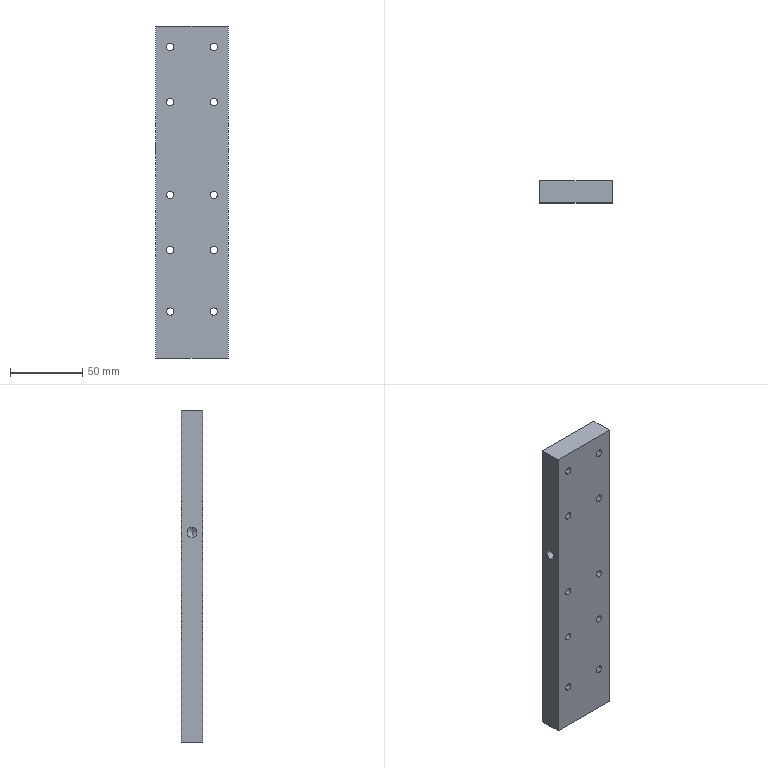Part | 1 solid | 38 faces | box 50 x 15 x 229 mm | volume 166833 mm3 | cylinder 26 | cone 6 | plane 6 | commonest cylinder face diameters 5 x20 6.8 x6
STEP:
#1=CARTESIAN_POINT('',(15.,0.,-48.5));
#2=VERTEX_POINT('',#1);
#3=CARTESIAN_POINT('',(15.,0.,-43.5));
#4=VERTEX_POINT('',#3);
#5=CARTESIAN_POINT('',(15.,0.,-46.));
#6=DIRECTION('',(0.,1.,0.));
#7=DIRECTION('',(0.,0.,1.));
#8=AXIS2_PLACEMENT_3D('',#5,#6,#7);
#9=CIRCLE('',#8,2.5);
#10=EDGE_CURVE('',#2,#4,#9,.T.);
#11=ORIENTED_EDGE('',*,*,#10,.F.);
#12=CARTESIAN_POINT('',(15.,15.,-48.5));
#13=VERTEX_POINT('',#12);
#14=CARTESIAN_POINT('',(15.,15.,-48.5));
#15=DIRECTION('',(0.,1.,0.));
#16=VECTOR('',#15,1000.);
#17=LINE('',#14,#16);
#18=EDGE_CURVE('',#2,#13,#17,.T.);
#19=ORIENTED_EDGE('',*,*,#18,.T.);
#20=CARTESIAN_POINT('',(15.,15.,-43.5));
#21=VERTEX_POINT('',#20);
#22=CARTESIAN_POINT('',(15.,15.,-46.));
#23=DIRECTION('',(0.,1.,0.));
#24=DIRECTION('',(0.,0.,1.));
#25=AXIS2_PLACEMENT_3D('',#22,#23,#24);
#26=CIRCLE('',#25,2.5);
#27=EDGE_CURVE('',#13,#21,#26,.T.);
#28=ORIENTED_EDGE('',*,*,#27,.T.);
#29=CARTESIAN_POINT('',(15.,15.,-43.5));
#30=DIRECTION('',(0.,1.,0.));
#31=VECTOR('',#30,1000.);
#32=LINE('',#29,#31);
#33=EDGE_CURVE('',#4,#21,#32,.T.);
#34=ORIENTED_EDGE('',*,*,#33,.F.);
#35=EDGE_LOOP('',(#11,#19,#28,#34));
#36=FACE_OUTER_BOUND('',#35,.T.);
#37=CARTESIAN_POINT('',(15.,15.,-46.));
#38=DIRECTION('',(0.,1.,0.));
#39=DIRECTION('',(0.,0.,1.));
#40=AXIS2_PLACEMENT_3D('',#37,#38,#39);
#41=CYLINDRICAL_SURFACE('',#40,2.5);
#42=ADVANCED_FACE('',(#36),#41,.F.);
#43=CARTESIAN_POINT('',(-15.,0.,-48.5));
#44=VERTEX_POINT('',#43);
#45=CARTESIAN_POINT('',(-15.,0.,-43.5));
#46=VERTEX_POINT('',#45);
#47=CARTESIAN_POINT('',(-15.,0.,-46.));
#48=DIRECTION('',(0.,1.,0.));
#49=DIRECTION('',(0.,0.,1.));
#50=AXIS2_PLACEMENT_3D('',#47,#48,#49);
#51=CIRCLE('',#50,2.5);
#52=EDGE_CURVE('',#44,#46,#51,.T.);
#53=ORIENTED_EDGE('',*,*,#52,.F.);
#54=CARTESIAN_POINT('',(-15.,15.,-48.5));
#55=VERTEX_POINT('',#54);
#56=CARTESIAN_POINT('',(-15.,15.,-48.5));
#57=DIRECTION('',(0.,1.,0.));
#58=VECTOR('',#57,1000.);
#59=LINE('',#56,#58);
#60=EDGE_CURVE('',#44,#55,#59,.T.);
#61=ORIENTED_EDGE('',*,*,#60,.T.);
#62=CARTESIAN_POINT('',(-15.,15.,-43.5));
#63=VERTEX_POINT('',#62);
#64=CARTESIAN_POINT('',(-15.,15.,-46.));
#65=DIRECTION('',(0.,1.,0.));
#66=DIRECTION('',(0.,0.,1.));
#67=AXIS2_PLACEMENT_3D('',#64,#65,#66);
#68=CIRCLE('',#67,2.5);
#69=EDGE_CURVE('',#55,#63,#68,.T.);
#70=ORIENTED_EDGE('',*,*,#69,.T.);
#71=CARTESIAN_POINT('',(-15.,15.,-43.5));
#72=DIRECTION('',(0.,1.,0.));
#73=VECTOR('',#72,1000.);
#74=LINE('',#71,#73);
#75=EDGE_CURVE('',#46,#63,#74,.T.);
#76=ORIENTED_EDGE('',*,*,#75,.F.);
#77=EDGE_LOOP('',(#53,#61,#70,#76));
#78=FACE_OUTER_BOUND('',#77,.T.);
#79=CARTESIAN_POINT('',(-15.,15.,-46.));
#80=DIRECTION('',(0.,1.,0.));
#81=DIRECTION('',(0.,0.,1.));
#82=AXIS2_PLACEMENT_3D('',#79,#80,#81);
#83=CYLINDRICAL_SURFACE('',#82,2.5);
#84=ADVANCED_FACE('',(#78),#83,.F.);
#85=CARTESIAN_POINT('',(-15.,0.,-10.5));
#86=VERTEX_POINT('',#85);
#87=CARTESIAN_POINT('',(-15.,0.,-5.5));
#88=VERTEX_POINT('',#87);
#89=CARTESIAN_POINT('',(-15.,0.,-8.));
#90=DIRECTION('',(0.,1.,0.));
#91=DIRECTION('',(0.,0.,1.));
#92=AXIS2_PLACEMENT_3D('',#89,#90,#91);
#93=CIRCLE('',#92,2.5);
#94=EDGE_CURVE('',#86,#88,#93,.T.);
#95=ORIENTED_EDGE('',*,*,#94,.F.);
#96=CARTESIAN_POINT('',(-15.,15.,-10.5));
#97=VERTEX_POINT('',#96);
#98=CARTESIAN_POINT('',(-15.,15.,-10.5));
#99=DIRECTION('',(0.,1.,0.));
#100=VECTOR('',#99,1000.);
#101=LINE('',#98,#100);
#102=EDGE_CURVE('',#86,#97,#101,.T.);
#103=ORIENTED_EDGE('',*,*,#102,.T.);
#104=CARTESIAN_POINT('',(-15.,15.,-5.5));
#105=VERTEX_POINT('',#104);
#106=CARTESIAN_POINT('',(-15.,15.,-8.));
#107=DIRECTION('',(0.,1.,0.));
#108=DIRECTION('',(0.,0.,1.));
#109=AXIS2_PLACEMENT_3D('',#106,#107,#108);
#110=CIRCLE('',#109,2.5);
#111=EDGE_CURVE('',#97,#105,#110,.T.);
#112=ORIENTED_EDGE('',*,*,#111,.T.);
#113=CARTESIAN_POINT('',(-15.,15.,-5.5));
#114=DIRECTION('',(0.,1.,0.));
#115=VECTOR('',#114,1000.);
#116=LINE('',#113,#115);
#117=EDGE_CURVE('',#88,#105,#116,.T.);
#118=ORIENTED_EDGE('',*,*,#117,.F.);
#119=EDGE_LOOP('',(#95,#103,#112,#118));
#120=FACE_OUTER_BOUND('',#119,.T.);
#121=CARTESIAN_POINT('',(-15.,15.,-8.));
#122=DIRECTION('',(0.,1.,0.));
#123=DIRECTION('',(0.,0.,1.));
#124=AXIS2_PLACEMENT_3D('',#121,#122,#123);
#125=CYLINDRICAL_SURFACE('',#124,2.5);
#126=ADVANCED_FACE('',(#120),#125,.F.);
#127=CARTESIAN_POINT('',(15.,0.,-10.5));
#128=VERTEX_POINT('',#127);
#129=CARTESIAN_POINT('',(15.,0.,-5.5));
#130=VERTEX_POINT('',#129);
#131=CARTESIAN_POINT('',(15.,0.,-8.));
#132=DIRECTION('',(0.,1.,0.));
#133=DIRECTION('',(0.,0.,1.));
#134=AXIS2_PLACEMENT_3D('',#131,#132,#133);
#135=CIRCLE('',#134,2.5);
#136=EDGE_CURVE('',#128,#130,#135,.T.);
#137=ORIENTED_EDGE('',*,*,#136,.F.);
#138=CARTESIAN_POINT('',(15.,15.,-10.5));
#139=VERTEX_POINT('',#138);
#140=CARTESIAN_POINT('',(15.,15.,-10.5));
#141=DIRECTION('',(0.,1.,0.));
#142=VECTOR('',#141,1000.);
#143=LINE('',#140,#142);
#144=EDGE_CURVE('',#128,#139,#143,.T.);
#145=ORIENTED_EDGE('',*,*,#144,.T.);
#146=CARTESIAN_POINT('',(15.,15.,-5.5));
#147=VERTEX_POINT('',#146);
#148=CARTESIAN_POINT('',(15.,15.,-8.));
#149=DIRECTION('',(0.,1.,0.));
#150=DIRECTION('',(0.,0.,1.));
#151=AXIS2_PLACEMENT_3D('',#148,#149,#150);
#152=CIRCLE('',#151,2.5);
#153=EDGE_CURVE('',#139,#147,#152,.T.);
#154=ORIENTED_EDGE('',*,*,#153,.T.);
#155=CARTESIAN_POINT('',(15.,15.,-5.5));
#156=DIRECTION('',(0.,1.,0.));
#157=VECTOR('',#156,1000.);
#158=LINE('',#155,#157);
#159=EDGE_CURVE('',#130,#147,#158,.T.);
#160=ORIENTED_EDGE('',*,*,#159,.F.);
#161=EDGE_LOOP('',(#137,#145,#154,#160));
#162=FACE_OUTER_BOUND('',#161,.T.);
#163=CARTESIAN_POINT('',(15.,15.,-8.));
#164=DIRECTION('',(0.,1.,0.));
#165=DIRECTION('',(0.,0.,1.));
#166=AXIS2_PLACEMENT_3D('',#163,#164,#165);
#167=CYLINDRICAL_SURFACE('',#166,2.5);
#168=ADVANCED_FACE('',(#162),#167,.F.);
#169=CARTESIAN_POINT('',(15.,0.,53.5));
#170=VERTEX_POINT('',#169);
#171=CARTESIAN_POINT('',(15.,0.,58.5));
#172=VERTEX_POINT('',#171);
#173=CARTESIAN_POINT('',(15.,0.,56.));
#174=DIRECTION('',(0.,1.,0.));
#175=DIRECTION('',(0.,0.,1.));
#176=AXIS2_PLACEMENT_3D('',#173,#174,#175);
#177=CIRCLE('',#176,2.5);
#178=EDGE_CURVE('',#170,#172,#177,.T.);
#179=ORIENTED_EDGE('',*,*,#178,.F.);
#180=CARTESIAN_POINT('',(15.,15.,53.5));
#181=VERTEX_POINT('',#180);
#182=CARTESIAN_POINT('',(15.,15.,53.5));
#183=DIRECTION('',(0.,1.,0.));
#184=VECTOR('',#183,1000.);
#185=LINE('',#182,#184);
#186=EDGE_CURVE('',#170,#181,#185,.T.);
#187=ORIENTED_EDGE('',*,*,#186,.T.);
#188=CARTESIAN_POINT('',(15.,15.,58.5));
#189=VERTEX_POINT('',#188);
#190=CARTESIAN_POINT('',(15.,15.,56.));
#191=DIRECTION('',(0.,1.,0.));
#192=DIRECTION('',(0.,0.,1.));
#193=AXIS2_PLACEMENT_3D('',#190,#191,#192);
#194=CIRCLE('',#193,2.5);
#195=EDGE_CURVE('',#181,#189,#194,.T.);
#196=ORIENTED_EDGE('',*,*,#195,.T.);
#197=CARTESIAN_POINT('',(15.,15.,58.5));
#198=DIRECTION('',(0.,1.,0.));
#199=VECTOR('',#198,1000.);
#200=LINE('',#197,#199);
#201=EDGE_CURVE('',#172,#189,#200,.T.);
#202=ORIENTED_EDGE('',*,*,#201,.F.);
#203=EDGE_LOOP('',(#179,#187,#196,#202));
#204=FACE_OUTER_BOUND('',#203,.T.);
#205=CARTESIAN_POINT('',(15.,15.,56.));
#206=DIRECTION('',(0.,1.,0.));
#207=DIRECTION('',(0.,0.,1.));
#208=AXIS2_PLACEMENT_3D('',#205,#206,#207);
#209=CYLINDRICAL_SURFACE('',#208,2.5);
#210=ADVANCED_FACE('',(#204),#209,.F.);
#211=CARTESIAN_POINT('',(-15.,0.,53.5));
#212=VERTEX_POINT('',#211);
#213=CARTESIAN_POINT('',(-15.,0.,58.5));
#214=VERTEX_POINT('',#213);
#215=CARTESIAN_POINT('',(-15.,0.,56.));
#216=DIRECTION('',(0.,1.,0.));
#217=DIRECTION('',(0.,0.,1.));
#218=AXIS2_PLACEMENT_3D('',#215,#216,#217);
#219=CIRCLE('',#218,2.5);
#220=EDGE_CURVE('',#212,#214,#219,.T.);
#221=ORIENTED_EDGE('',*,*,#220,.F.);
#222=CARTESIAN_POINT('',(-15.,15.,53.5));
#223=VERTEX_POINT('',#222);
#224=CARTESIAN_POINT('',(-15.,15.,53.5));
#225=DIRECTION('',(0.,1.,0.));
#226=VECTOR('',#225,1000.);
#227=LINE('',#224,#226);
#228=EDGE_CURVE('',#212,#223,#227,.T.);
#229=ORIENTED_EDGE('',*,*,#228,.T.);
#230=CARTESIAN_POINT('',(-15.,15.,58.5));
#231=VERTEX_POINT('',#230);
#232=CARTESIAN_POINT('',(-15.,15.,56.));
#233=DIRECTION('',(0.,1.,0.));
#234=DIRECTION('',(0.,0.,1.));
#235=AXIS2_PLACEMENT_3D('',#232,#233,#234);
#236=CIRCLE('',#235,2.5);
#237=EDGE_CURVE('',#223,#231,#236,.T.);
#238=ORIENTED_EDGE('',*,*,#237,.T.);
#239=CARTESIAN_POINT('',(-15.,15.,58.5));
#240=DIRECTION('',(0.,1.,0.));
#241=VECTOR('',#240,1000.);
#242=LINE('',#239,#241);
#243=EDGE_CURVE('',#214,#231,#242,.T.);
#244=ORIENTED_EDGE('',*,*,#243,.F.);
#245=EDGE_LOOP('',(#221,#229,#238,#244));
#246=FACE_OUTER_BOUND('',#245,.T.);
#247=CARTESIAN_POINT('',(-15.,15.,56.));
#248=DIRECTION('',(0.,1.,0.));
#249=DIRECTION('',(0.,0.,1.));
#250=AXIS2_PLACEMENT_3D('',#247,#248,#249);
#251=CYLINDRICAL_SURFACE('',#250,2.5);
#252=ADVANCED_FACE('',(#246),#251,.F.);
#253=CARTESIAN_POINT('',(15.,0.,91.5));
#254=VERTEX_POINT('',#253);
#255=CARTESIAN_POINT('',(15.,0.,96.5));
#256=VERTEX_POINT('',#255);
#257=CARTESIAN_POINT('',(15.,0.,94.));
#258=DIRECTION('',(0.,1.,0.));
#259=DIRECTION('',(0.,0.,1.));
#260=AXIS2_PLACEMENT_3D('',#257,#258,#259);
#261=CIRCLE('',#260,2.5);
#262=EDGE_CURVE('',#254,#256,#261,.T.);
#263=ORIENTED_EDGE('',*,*,#262,.F.);
#264=CARTESIAN_POINT('',(15.,15.,91.5));
#265=VERTEX_POINT('',#264);
#266=CARTESIAN_POINT('',(15.,15.,91.5));
#267=DIRECTION('',(0.,1.,0.));
#268=VECTOR('',#267,1000.);
#269=LINE('',#266,#268);
#270=EDGE_CURVE('',#254,#265,#269,.T.);
#271=ORIENTED_EDGE('',*,*,#270,.T.);
#272=CARTESIAN_POINT('',(15.,15.,96.5));
#273=VERTEX_POINT('',#272);
#274=CARTESIAN_POINT('',(15.,15.,94.));
#275=DIRECTION('',(0.,1.,0.));
#276=DIRECTION('',(0.,0.,1.));
#277=AXIS2_PLACEMENT_3D('',#274,#275,#276);
#278=CIRCLE('',#277,2.5);
#279=EDGE_CURVE('',#265,#273,#278,.T.);
#280=ORIENTED_EDGE('',*,*,#279,.T.);
#281=CARTESIAN_POINT('',(15.,15.,96.5));
#282=DIRECTION('',(0.,1.,0.));
#283=VECTOR('',#282,1000.);
#284=LINE('',#281,#283);
#285=EDGE_CURVE('',#256,#273,#284,.T.);
#286=ORIENTED_EDGE('',*,*,#285,.F.);
#287=EDGE_LOOP('',(#263,#271,#280,#286));
#288=FACE_OUTER_BOUND('',#287,.T.);
#289=CARTESIAN_POINT('',(15.,15.,94.));
#290=DIRECTION('',(0.,1.,0.));
#291=DIRECTION('',(0.,0.,1.));
#292=AXIS2_PLACEMENT_3D('',#289,#290,#291);
#293=CYLINDRICAL_SURFACE('',#292,2.5);
#294=ADVANCED_FACE('',(#288),#293,.F.);
#295=CARTESIAN_POINT('',(-15.,0.,91.5));
#296=VERTEX_POINT('',#295);
#297=CARTESIAN_POINT('',(-15.,0.,96.5));
#298=VERTEX_POINT('',#297);
#299=CARTESIAN_POINT('',(-15.,0.,94.));
#300=DIRECTION('',(0.,1.,0.));
#301=DIRECTION('',(0.,0.,1.));
#302=AXIS2_PLACEMENT_3D('',#299,#300,#301);
#303=CIRCLE('',#302,2.5);
#304=EDGE_CURVE('',#296,#298,#303,.T.);
#305=ORIENTED_EDGE('',*,*,#304,.F.);
#306=CARTESIAN_POINT('',(-15.,15.,91.5));
#307=VERTEX_POINT('',#306);
#308=CARTESIAN_POINT('',(-15.,15.,91.5));
#309=DIRECTION('',(0.,1.,0.));
#310=VECTOR('',#309,1000.);
#311=LINE('',#308,#310);
#312=EDGE_CURVE('',#296,#307,#311,.T.);
#313=ORIENTED_EDGE('',*,*,#312,.T.);
#314=CARTESIAN_POINT('',(-15.,15.,96.5));
#315=VERTEX_POINT('',#314);
#316=CARTESIAN_POINT('',(-15.,15.,94.));
#317=DIRECTION('',(0.,1.,0.));
#318=DIRECTION('',(0.,0.,1.));
#319=AXIS2_PLACEMENT_3D('',#316,#317,#318);
#320=CIRCLE('',#319,2.5);
#321=EDGE_CURVE('',#307,#315,#320,.T.);
#322=ORIENTED_EDGE('',*,*,#321,.T.);
#323=CARTESIAN_POINT('',(-15.,15.,96.5));
#324=DIRECTION('',(0.,1.,0.));
#325=VECTOR('',#324,1000.);
#326=LINE('',#323,#325);
#327=EDGE_CURVE('',#298,#315,#326,.T.);
#328=ORIENTED_EDGE('',*,*,#327,.F.);
#329=EDGE_LOOP('',(#305,#313,#322,#328));
#330=FACE_OUTER_BOUND('',#329,.T.);
#331=CARTESIAN_POINT('',(-15.,15.,94.));
#332=DIRECTION('',(0.,1.,0.));
#333=DIRECTION('',(0.,0.,1.));
#334=AXIS2_PLACEMENT_3D('',#331,#332,#333);
#335=CYLINDRICAL_SURFACE('',#334,2.5);
#336=ADVANCED_FACE('',(#330),#335,.F.);
#337=CARTESIAN_POINT('',(15.,0.,-91.));
#338=VERTEX_POINT('',#337);
#339=CARTESIAN_POINT('',(15.,0.,-86.));
#340=VERTEX_POINT('',#339);
#341=CARTESIAN_POINT('',(15.,0.,-88.5));
#342=DIRECTION('',(0.,1.,0.));
#343=DIRECTION('',(0.,0.,1.));
#344=AXIS2_PLACEMENT_3D('',#341,#342,#343);
#345=CIRCLE('',#344,2.5);
#346=EDGE_CURVE('',#338,#340,#345,.T.);
#347=ORIENTED_EDGE('',*,*,#346,.F.);
#348=CARTESIAN_POINT('',(15.,15.,-91.));
#349=VERTEX_POINT('',#348);
#350=CARTESIAN_POINT('',(15.,15.,-91.));
#351=DIRECTION('',(0.,1.,0.));
#352=VECTOR('',#351,1000.);
#353=LINE('',#350,#352);
#354=EDGE_CURVE('',#338,#349,#353,.T.);
#355=ORIENTED_EDGE('',*,*,#354,.T.);
#356=CARTESIAN_POINT('',(15.,15.,-86.));
#357=VERTEX_POINT('',#356);
#358=CARTESIAN_POINT('',(15.,15.,-88.5));
#359=DIRECTION('',(0.,1.,0.));
#360=DIRECTION('',(0.,0.,1.));
#361=AXIS2_PLACEMENT_3D('',#358,#359,#360);
#362=CIRCLE('',#361,2.5);
#363=EDGE_CURVE('',#349,#357,#362,.T.);
#364=ORIENTED_EDGE('',*,*,#363,.T.);
#365=CARTESIAN_POINT('',(15.,15.,-86.));
#366=DIRECTION('',(0.,1.,0.));
#367=VECTOR('',#366,1000.);
#368=LINE('',#365,#367);
#369=EDGE_CURVE('',#340,#357,#368,.T.);
#370=ORIENTED_EDGE('',*,*,#369,.F.);
#371=EDGE_LOOP('',(#347,#355,#364,#370));
#372=FACE_OUTER_BOUND('',#371,.T.);
#373=CARTESIAN_POINT('',(15.,15.,-88.5));
#374=DIRECTION('',(0.,1.,0.));
#375=DIRECTION('',(0.,0.,1.));
#376=AXIS2_PLACEMENT_3D('',#373,#374,#375);
#377=CYLINDRICAL_SURFACE('',#376,2.5);
#378=ADVANCED_FACE('',(#372),#377,.F.);
#379=CARTESIAN_POINT('',(-15.,0.,-91.));
#380=VERTEX_POINT('',#379);
#381=CARTESIAN_POINT('',(-15.,0.,-86.));
#382=VERTEX_POINT('',#381);
#383=CARTESIAN_POINT('',(-15.,0.,-88.5));
#384=DIRECTION('',(0.,1.,0.));
#385=DIRECTION('',(0.,0.,1.));
#386=AXIS2_PLACEMENT_3D('',#383,#384,#385);
#387=CIRCLE('',#386,2.5);
#388=EDGE_CURVE('',#380,#382,#387,.T.);
#389=ORIENTED_EDGE('',*,*,#388,.F.);
#390=CARTESIAN_POINT('',(-15.,15.,-91.));
#391=VERTEX_POINT('',#390);
#392=CARTESIAN_POINT('',(-15.,15.,-91.));
#393=DIRECTION('',(0.,1.,0.));
#394=VECTOR('',#393,1000.);
#395=LINE('',#392,#394);
#396=EDGE_CURVE('',#380,#391,#395,.T.);
#397=ORIENTED_EDGE('',*,*,#396,.T.);
#398=CARTESIAN_POINT('',(-15.,15.,-86.));
#399=VERTEX_POINT('',#398);
#400=CARTESIAN_POINT('',(-15.,15.,-88.5));
#401=DIRECTION('',(0.,1.,0.));
#402=DIRECTION('',(0.,0.,1.));
#403=AXIS2_PLACEMENT_3D('',#400,#401,#402);
#404=CIRCLE('',#403,2.5);
#405=EDGE_CURVE('',#391,#399,#404,.T.);
#406=ORIENTED_EDGE('',*,*,#405,.T.);
#407=CARTESIAN_POINT('',(-15.,15.,-86.));
#408=DIRECTION('',(0.,1.,0.));
#409=VECTOR('',#408,1000.);
#410=LINE('',#407,#409);
#411=EDGE_CURVE('',#382,#399,#410,.T.);
#412=ORIENTED_EDGE('',*,*,#411,.F.);
#413=EDGE_LOOP('',(#389,#397,#406,#412));
#414=FACE_OUTER_BOUND('',#413,.T.);
#415=CARTESIAN_POINT('',(-15.,15.,-88.5));
#416=DIRECTION('',(0.,1.,0.));
#417=DIRECTION('',(0.,0.,1.));
#418=AXIS2_PLACEMENT_3D('',#415,#416,#417);
#419=CYLINDRICAL_SURFACE('',#418,2.5);
#420=ADVANCED_FACE('',(#414),#419,.F.);
#421=CARTESIAN_POINT('',(-2.75,7.5,20.7));
#422=VERTEX_POINT('',#421);
#423=CARTESIAN_POINT('',(-2.75,7.5,27.5));
#424=VERTEX_POINT('',#423);
#425=CARTESIAN_POINT('',(-2.75,7.5,24.1));
#426=DIRECTION('',(-1.,0.,0.));
#427=DIRECTION('',(0.,0.,1.));
#428=AXIS2_PLACEMENT_3D('',#425,#426,#427);
#429=CIRCLE('',#428,3.4);
#430=EDGE_CURVE('',#422,#424,#429,.T.);
#431=ORIENTED_EDGE('',*,*,#430,.F.);
#432=CARTESIAN_POINT('',(-25.,7.5,20.7));
#433=VERTEX_POINT('',#432);
#434=CARTESIAN_POINT('',(-25.,7.5,20.7));
#435=DIRECTION('',(-1.,0.,0.));
#436=VECTOR('',#435,1000.);
#437=LINE('',#434,#436);
#438=EDGE_CURVE('',#422,#433,#437,.T.);
#439=ORIENTED_EDGE('',*,*,#438,.T.);
#440=CARTESIAN_POINT('',(-25.,7.5,27.5));
#441=VERTEX_POINT('',#440);
#442=CARTESIAN_POINT('',(-25.,7.5,24.1));
#443=DIRECTION('',(-1.,0.,0.));
#444=DIRECTION('',(0.,0.,1.));
#445=AXIS2_PLACEMENT_3D('',#442,#443,#444);
#446=CIRCLE('',#445,3.4);
#447=EDGE_CURVE('',#433,#441,#446,.T.);
#448=ORIENTED_EDGE('',*,*,#447,.T.);
#449=CARTESIAN_POINT('',(-25.,7.5,27.5));
#450=DIRECTION('',(-1.,0.,0.));
#451=VECTOR('',#450,1000.);
#452=LINE('',#449,#451);
#453=EDGE_CURVE('',#424,#441,#452,.T.);
#454=ORIENTED_EDGE('',*,*,#453,.F.);
#455=EDGE_LOOP('',(#431,#439,#448,#454));
#456=FACE_OUTER_BOUND('',#455,.T.);
#457=CARTESIAN_POINT('',(-25.,7.5,24.1));
#458=DIRECTION('',(-1.,0.,0.));
#459=DIRECTION('',(0.,0.,1.));
#460=AXIS2_PLACEMENT_3D('',#457,#458,#459);
#461=CYLINDRICAL_SURFACE('',#460,3.4);
#462=ADVANCED_FACE('',(#456),#461,.F.);
#463=CARTESIAN_POINT('',(-0.7071,7.5,24.1));
#464=VERTEX_POINT('',#463);
#465=CARTESIAN_POINT('',(-2.75,7.5,27.5));
#466=DIRECTION('',(-0.515,0.,0.8572));
#467=VECTOR('',#466,1000.);
#468=LINE('',#465,#467);
#469=EDGE_CURVE('',#464,#424,#468,.T.);
#470=ORIENTED_EDGE('',*,*,#469,.F.);
#471=CARTESIAN_POINT('',(-2.75,7.5,20.7));
#472=DIRECTION('',(-0.515,0.,-0.8572));
#473=VECTOR('',#472,1000.);
#474=LINE('',#471,#473);
#475=EDGE_CURVE('',#464,#422,#474,.T.);
#476=ORIENTED_EDGE('',*,*,#475,.T.);
#477=ORIENTED_EDGE('',*,*,#430,.T.);
#478=EDGE_LOOP('',(#470,#476,#477));
#479=FACE_OUTER_BOUND('',#478,.T.);
#480=CARTESIAN_POINT('',(-2.75,7.5,24.1));
#481=DIRECTION('',(-1.,0.,0.));
#482=DIRECTION('',(0.,0.,1.));
#483=AXIS2_PLACEMENT_3D('',#480,#481,#482);
#484=CONICAL_SURFACE('',#483,3.4,1.03);
#485=ADVANCED_FACE('',(#479),#484,.F.);
#486=CARTESIAN_POINT('',(-11.6,7.5,-105.5));
#487=VERTEX_POINT('',#486);
#488=CARTESIAN_POINT('',(-18.4,7.5,-105.5));
#489=VERTEX_POINT('',#488);
#490=CARTESIAN_POINT('',(-15.,7.5,-105.5));
#491=DIRECTION('',(0.,0.,-1.));
#492=DIRECTION('',(-1.,0.,0.));
#493=AXIS2_PLACEMENT_3D('',#490,#491,#492);
#494=CIRCLE('',#493,3.4);
#495=EDGE_CURVE('',#487,#489,#494,.T.);
#496=ORIENTED_EDGE('',*,*,#495,.F.);
#497=CARTESIAN_POINT('',(-11.6,7.5,-120.5));
#498=VERTEX_POINT('',#497);
#499=CARTESIAN_POINT('',(-11.6,7.5,-120.5));
#500=DIRECTION('',(0.,0.,-1.));
#501=VECTOR('',#500,1000.);
#502=LINE('',#499,#501);
#503=EDGE_CURVE('',#487,#498,#502,.T.);
#504=ORIENTED_EDGE('',*,*,#503,.T.);
#505=CARTESIAN_POINT('',(-18.4,7.5,-120.5));
#506=VERTEX_POINT('',#505);
#507=CARTESIAN_POINT('',(-15.,7.5,-120.5));
#508=DIRECTION('',(0.,0.,-1.));
#509=DIRECTION('',(-1.,0.,0.));
#510=AXIS2_PLACEMENT_3D('',#507,#508,#509);
#511=CIRCLE('',#510,3.4);
#512=EDGE_CURVE('',#498,#506,#511,.T.);
#513=ORIENTED_EDGE('',*,*,#512,.T.);
#514=CARTESIAN_POINT('',(-18.4,7.5,-120.5));
#515=DIRECTION('',(0.,0.,-1.));
#516=VECTOR('',#515,1000.);
#517=LINE('',#514,#516);
#518=EDGE_CURVE('',#489,#506,#517,.T.);
#519=ORIENTED_EDGE('',*,*,#518,.F.);
#520=EDGE_LOOP('',(#496,#504,#513,#519));
#521=FACE_OUTER_BOUND('',#520,.T.);
#522=CARTESIAN_POINT('',(-15.,7.5,-120.5));
#523=DIRECTION('',(0.,0.,-1.));
#524=DIRECTION('',(-1.,0.,0.));
#525=AXIS2_PLACEMENT_3D('',#522,#523,#524);
#526=CYLINDRICAL_SURFACE('',#525,3.4);
#527=ADVANCED_FACE('',(#521),#526,.F.);
#528=CARTESIAN_POINT('',(-15.,7.5,-103.457));
#529=VERTEX_POINT('',#528);
#530=CARTESIAN_POINT('',(-18.4,7.5,-105.5));
#531=DIRECTION('',(-0.8572,0.,-0.515));
#532=VECTOR('',#531,1000.);
#533=LINE('',#530,#532);
#534=EDGE_CURVE('',#529,#489,#533,.T.);
#535=ORIENTED_EDGE('',*,*,#534,.F.);
#536=CARTESIAN_POINT('',(-11.6,7.5,-105.5));
#537=DIRECTION('',(0.8572,0.,-0.515));
#538=VECTOR('',#537,1000.);
#539=LINE('',#536,#538);
#540=EDGE_CURVE('',#529,#487,#539,.T.);
#541=ORIENTED_EDGE('',*,*,#540,.T.);
#542=ORIENTED_EDGE('',*,*,#495,.T.);
#543=EDGE_LOOP('',(#535,#541,#542));
#544=FACE_OUTER_BOUND('',#543,.T.);
#545=CARTESIAN_POINT('',(-15.,7.5,-105.5));
#546=DIRECTION('',(0.,0.,-1.));
#547=DIRECTION('',(-1.,0.,0.));
#548=AXIS2_PLACEMENT_3D('',#545,#546,#547);
#549=CONICAL_SURFACE('',#548,3.4,1.03);
#550=ADVANCED_FACE('',(#544),#549,.F.);
#551=CARTESIAN_POINT('',(18.4,7.5,-105.5));
#552=VERTEX_POINT('',#551);
#553=CARTESIAN_POINT('',(11.6,7.5,-105.5));
#554=VERTEX_POINT('',#553);
#555=CARTESIAN_POINT('',(15.,7.5,-105.5));
#556=DIRECTION('',(0.,0.,-1.));
#557=DIRECTION('',(-1.,0.,0.));
#558=AXIS2_PLACEMENT_3D('',#555,#556,#557);
#559=CIRCLE('',#558,3.4);
#560=EDGE_CURVE('',#552,#554,#559,.T.);
#561=ORIENTED_EDGE('',*,*,#560,.F.);
#562=CARTESIAN_POINT('',(18.4,7.5,-120.5));
#563=VERTEX_POINT('',#562);
#564=CARTESIAN_POINT('',(18.4,7.5,-120.5));
#565=DIRECTION('',(0.,0.,-1.));
#566=VECTOR('',#565,1000.);
#567=LINE('',#564,#566);
#568=EDGE_CURVE('',#552,#563,#567,.T.);
#569=ORIENTED_EDGE('',*,*,#568,.T.);
#570=CARTESIAN_POINT('',(11.6,7.5,-120.5));
#571=VERTEX_POINT('',#570);
#572=CARTESIAN_POINT('',(15.,7.5,-120.5));
#573=DIRECTION('',(0.,0.,-1.));
#574=DIRECTION('',(-1.,0.,0.));
#575=AXIS2_PLACEMENT_3D('',#572,#573,#574);
#576=CIRCLE('',#575,3.4);
#577=EDGE_CURVE('',#563,#571,#576,.T.);
#578=ORIENTED_EDGE('',*,*,#577,.T.);
#579=CARTESIAN_POINT('',(11.6,7.5,-120.5));
#580=DIRECTION('',(0.,0.,-1.));
#581=VECTOR('',#580,1000.);
#582=LINE('',#579,#581);
#583=EDGE_CURVE('',#554,#571,#582,.T.);
#584=ORIENTED_EDGE('',*,*,#583,.F.);
#585=EDGE_LOOP('',(#561,#569,#578,#584));
#586=FACE_OUTER_BOUND('',#585,.T.);
#587=CARTESIAN_POINT('',(15.,7.5,-120.5));
#588=DIRECTION('',(0.,0.,-1.));
#589=DIRECTION('',(-1.,0.,0.));
#590=AXIS2_PLACEMENT_3D('',#587,#588,#589);
#591=CYLINDRICAL_SURFACE('',#590,3.4);
#592=ADVANCED_FACE('',(#586),#591,.F.);
#593=CARTESIAN_POINT('',(15.,7.5,-103.457));
#594=VERTEX_POINT('',#593);
#595=CARTESIAN_POINT('',(11.6,7.5,-105.5));
#596=DIRECTION('',(-0.8572,0.,-0.515));
#597=VECTOR('',#596,1000.);
#598=LINE('',#595,#597);
#599=EDGE_CURVE('',#594,#554,#598,.T.);
#600=ORIENTED_EDGE('',*,*,#599,.F.);
#601=CARTESIAN_POINT('',(18.4,7.5,-105.5));
#602=DIRECTION('',(0.8572,0.,-0.515));
#603=VECTOR('',#602,1000.);
#604=LINE('',#601,#603);
#605=EDGE_CURVE('',#594,#552,#604,.T.);
#606=ORIENTED_EDGE('',*,*,#605,.T.);
#607=ORIENTED_EDGE('',*,*,#560,.T.);
#608=EDGE_LOOP('',(#600,#606,#607));
#609=FACE_OUTER_BOUND('',#608,.T.);
#610=CARTESIAN_POINT('',(15.,7.5,-105.5));
#611=DIRECTION('',(0.,0.,-1.));
#612=DIRECTION('',(-1.,0.,0.));
#613=AXIS2_PLACEMENT_3D('',#610,#611,#612);
#614=CONICAL_SURFACE('',#613,3.4,1.03);
#615=ADVANCED_FACE('',(#609),#614,.F.);
#616=CARTESIAN_POINT('',(-25.,15.,108.5));
#617=VERTEX_POINT('',#616);
#618=CARTESIAN_POINT('',(25.,15.,108.5));
#619=VERTEX_POINT('',#618);
#620=CARTESIAN_POINT('',(-25.,15.,108.5));
#621=DIRECTION('',(1.,0.,0.));
#622=VECTOR('',#621,1000.);
#623=LINE('',#620,#622);
#624=EDGE_CURVE('',#617,#619,#623,.T.);
#625=ORIENTED_EDGE('',*,*,#624,.F.);
#626=CARTESIAN_POINT('',(-25.,0.,108.5));
#627=VERTEX_POINT('',#626);
#628=CARTESIAN_POINT('',(-25.,0.,108.5));
#629=DIRECTION('',(0.,1.,0.));
#630=VECTOR('',#629,1000.);
#631=LINE('',#628,#630);
#632=EDGE_CURVE('',#627,#617,#631,.T.);
#633=ORIENTED_EDGE('',*,*,#632,.F.);
#634=CARTESIAN_POINT('',(25.,0.,108.5));
#635=VERTEX_POINT('',#634);
#636=CARTESIAN_POINT('',(-25.,0.,108.5));
#637=DIRECTION('',(1.,0.,0.));
#638=VECTOR('',#637,1000.);
#639=LINE('',#636,#638);
#640=EDGE_CURVE('',#627,#635,#639,.T.);
#641=ORIENTED_EDGE('',*,*,#640,.T.);
#642=CARTESIAN_POINT('',(25.,0.,108.5));
#643=DIRECTION('',(0.,1.,0.));
#644=VECTOR('',#643,1000.);
#645=LINE('',#642,#644);
#646=EDGE_CURVE('',#635,#619,#645,.T.);
#647=ORIENTED_EDGE('',*,*,#646,.T.);
#648=EDGE_LOOP('',(#625,#633,#641,#647));
#649=FACE_OUTER_BOUND('',#648,.T.);
#650=CARTESIAN_POINT('',(-25.,0.,108.5));
#651=DIRECTION('',(0.,0.,1.));
#652=DIRECTION('',(1.,0.,0.));
#653=AXIS2_PLACEMENT_3D('',#650,#651,#652);
#654=PLANE('',#653);
#655=ADVANCED_FACE('',(#649),#654,.T.);
#656=CARTESIAN_POINT('',(-25.,7.5,24.1));
#657=DIRECTION('',(-1.,0.,0.));
#658=DIRECTION('',(0.,0.,1.));
#659=AXIS2_PLACEMENT_3D('',#656,#657,#658);
#660=CIRCLE('',#659,3.4);
#661=EDGE_CURVE('',#441,#433,#660,.T.);
#662=ORIENTED_EDGE('',*,*,#661,.F.);
#663=ORIENTED_EDGE('',*,*,#447,.F.);
#664=EDGE_LOOP('',(#662,#663));
#665=FACE_BOUND('',#664,.T.);
#666=CARTESIAN_POINT('',(-25.,15.,-120.5));
#667=VERTEX_POINT('',#666);
#668=CARTESIAN_POINT('',(-25.,15.,-120.5));
#669=DIRECTION('',(0.,0.,1.));
#670=VECTOR('',#669,1000.);
#671=LINE('',#668,#670);
#672=EDGE_CURVE('',#667,#617,#671,.T.);
#673=ORIENTED_EDGE('',*,*,#672,.F.);
#674=CARTESIAN_POINT('',(-25.,0.,-120.5));
#675=VERTEX_POINT('',#674);
#676=CARTESIAN_POINT('',(-25.,0.,-120.5));
#677=DIRECTION('',(0.,1.,0.));
#678=VECTOR('',#677,1000.);
#679=LINE('',#676,#678);
#680=EDGE_CURVE('',#675,#667,#679,.T.);
#681=ORIENTED_EDGE('',*,*,#680,.F.);
#682=CARTESIAN_POINT('',(-25.,0.,-120.5));
#683=DIRECTION('',(0.,0.,1.));
#684=VECTOR('',#683,1000.);
#685=LINE('',#682,#684);
#686=EDGE_CURVE('',#675,#627,#685,.T.);
#687=ORIENTED_EDGE('',*,*,#686,.T.);
#688=ORIENTED_EDGE('',*,*,#632,.T.);
#689=EDGE_LOOP('',(#673,#681,#687,#688));
#690=FACE_OUTER_BOUND('',#689,.T.);
#691=CARTESIAN_POINT('',(-25.,0.,-120.5));
#692=DIRECTION('',(-1.,0.,0.));
#693=DIRECTION('',(0.,0.,1.));
#694=AXIS2_PLACEMENT_3D('',#691,#692,#693);
#695=PLANE('',#694);
#696=ADVANCED_FACE('',(#665,#690),#695,.T.);
#697=CARTESIAN_POINT('',(-15.,7.5,-120.5));
#698=DIRECTION('',(0.,0.,-1.));
#699=DIRECTION('',(-1.,0.,0.));
#700=AXIS2_PLACEMENT_3D('',#697,#698,#699);
#701=CIRCLE('',#700,3.4);
#702=EDGE_CURVE('',#506,#498,#701,.T.);
#703=ORIENTED_EDGE('',*,*,#702,.F.);
#704=ORIENTED_EDGE('',*,*,#512,.F.);
#705=EDGE_LOOP('',(#703,#704));
#706=FACE_BOUND('',#705,.T.);
#707=CARTESIAN_POINT('',(15.,7.5,-120.5));
#708=DIRECTION('',(0.,0.,-1.));
#709=DIRECTION('',(-1.,0.,0.));
#710=AXIS2_PLACEMENT_3D('',#707,#708,#709);
#711=CIRCLE('',#710,3.4);
#712=EDGE_CURVE('',#571,#563,#711,.T.);
#713=ORIENTED_EDGE('',*,*,#712,.F.);
#714=ORIENTED_EDGE('',*,*,#577,.F.);
#715=EDGE_LOOP('',(#713,#714));
#716=FACE_BOUND('',#715,.T.);
#717=CARTESIAN_POINT('',(25.,15.,-120.5));
#718=VERTEX_POINT('',#717);
#719=CARTESIAN_POINT('',(25.,15.,-120.5));
#720=DIRECTION('',(-1.,0.,0.));
#721=VECTOR('',#720,1000.);
#722=LINE('',#719,#721);
#723=EDGE_CURVE('',#718,#667,#722,.T.);
#724=ORIENTED_EDGE('',*,*,#723,.F.);
#725=CARTESIAN_POINT('',(25.,0.,-120.5));
#726=VERTEX_POINT('',#725);
#727=CARTESIAN_POINT('',(25.,0.,-120.5));
#728=DIRECTION('',(0.,1.,0.));
#729=VECTOR('',#728,1000.);
#730=LINE('',#727,#729);
#731=EDGE_CURVE('',#726,#718,#730,.T.);
#732=ORIENTED_EDGE('',*,*,#731,.F.);
#733=CARTESIAN_POINT('',(25.,0.,-120.5));
#734=DIRECTION('',(-1.,0.,0.));
#735=VECTOR('',#734,1000.);
#736=LINE('',#733,#735);
#737=EDGE_CURVE('',#726,#675,#736,.T.);
#738=ORIENTED_EDGE('',*,*,#737,.T.);
#739=ORIENTED_EDGE('',*,*,#680,.T.);
#740=EDGE_LOOP('',(#724,#732,#738,#739));
#741=FACE_OUTER_BOUND('',#740,.T.);
#742=CARTESIAN_POINT('',(25.,0.,-120.5));
#743=DIRECTION('',(0.,0.,-1.));
#744=DIRECTION('',(-1.,0.,0.));
#745=AXIS2_PLACEMENT_3D('',#742,#743,#744);
#746=PLANE('',#745);
#747=ADVANCED_FACE('',(#706,#716,#741),#746,.T.);
#748=CARTESIAN_POINT('',(25.,15.,108.5));
#749=DIRECTION('',(0.,0.,-1.));
#750=VECTOR('',#749,1000.);
#751=LINE('',#748,#750);
#752=EDGE_CURVE('',#619,#718,#751,.T.);
#753=ORIENTED_EDGE('',*,*,#752,.F.);
#754=ORIENTED_EDGE('',*,*,#646,.F.);
#755=CARTESIAN_POINT('',(25.,0.,108.5));
#756=DIRECTION('',(0.,0.,-1.));
#757=VECTOR('',#756,1000.);
#758=LINE('',#755,#757);
#759=EDGE_CURVE('',#635,#726,#758,.T.);
#760=ORIENTED_EDGE('',*,*,#759,.T.);
#761=ORIENTED_EDGE('',*,*,#731,.T.);
#762=EDGE_LOOP('',(#753,#754,#760,#761));
#763=FACE_OUTER_BOUND('',#762,.T.);
#764=CARTESIAN_POINT('',(25.,0.,108.5));
#765=DIRECTION('',(1.,0.,0.));
#766=DIRECTION('',(0.,0.,-1.));
#767=AXIS2_PLACEMENT_3D('',#764,#765,#766);
#768=PLANE('',#767);
#769=ADVANCED_FACE('',(#763),#768,.T.);
#770=CARTESIAN_POINT('',(15.,0.,-46.));
#771=DIRECTION('',(0.,1.,0.));
#772=DIRECTION('',(0.,0.,1.));
#773=AXIS2_PLACEMENT_3D('',#770,#771,#772);
#774=CIRCLE('',#773,2.5);
#775=EDGE_CURVE('',#4,#2,#774,.T.);
#776=ORIENTED_EDGE('',*,*,#775,.T.);
#777=ORIENTED_EDGE('',*,*,#10,.T.);
#778=EDGE_LOOP('',(#776,#777));
#779=FACE_BOUND('',#778,.T.);
#780=CARTESIAN_POINT('',(-15.,0.,-46.));
#781=DIRECTION('',(0.,1.,0.));
#782=DIRECTION('',(0.,0.,1.));
#783=AXIS2_PLACEMENT_3D('',#780,#781,#782);
#784=CIRCLE('',#783,2.5);
#785=EDGE_CURVE('',#46,#44,#784,.T.);
#786=ORIENTED_EDGE('',*,*,#785,.T.);
#787=ORIENTED_EDGE('',*,*,#52,.T.);
#788=EDGE_LOOP('',(#786,#787));
#789=FACE_BOUND('',#788,.T.);
#790=CARTESIAN_POINT('',(-15.,0.,-8.));
#791=DIRECTION('',(0.,1.,0.));
#792=DIRECTION('',(0.,0.,1.));
#793=AXIS2_PLACEMENT_3D('',#790,#791,#792);
#794=CIRCLE('',#793,2.5);
#795=EDGE_CURVE('',#88,#86,#794,.T.);
#796=ORIENTED_EDGE('',*,*,#795,.T.);
#797=ORIENTED_EDGE('',*,*,#94,.T.);
#798=EDGE_LOOP('',(#796,#797));
#799=FACE_BOUND('',#798,.T.);
#800=CARTESIAN_POINT('',(15.,0.,-8.));
#801=DIRECTION('',(0.,1.,0.));
#802=DIRECTION('',(0.,0.,1.));
#803=AXIS2_PLACEMENT_3D('',#800,#801,#802);
#804=CIRCLE('',#803,2.5);
#805=EDGE_CURVE('',#130,#128,#804,.T.);
#806=ORIENTED_EDGE('',*,*,#805,.T.);
#807=ORIENTED_EDGE('',*,*,#136,.T.);
#808=EDGE_LOOP('',(#806,#807));
#809=FACE_BOUND('',#808,.T.);
#810=CARTESIAN_POINT('',(15.,0.,56.));
#811=DIRECTION('',(0.,1.,0.));
#812=DIRECTION('',(0.,0.,1.));
#813=AXIS2_PLACEMENT_3D('',#810,#811,#812);
#814=CIRCLE('',#813,2.5);
#815=EDGE_CURVE('',#172,#170,#814,.T.);
#816=ORIENTED_EDGE('',*,*,#815,.T.);
#817=ORIENTED_EDGE('',*,*,#178,.T.);
#818=EDGE_LOOP('',(#816,#817));
#819=FACE_BOUND('',#818,.T.);
#820=CARTESIAN_POINT('',(-15.,0.,56.));
#821=DIRECTION('',(0.,1.,0.));
#822=DIRECTION('',(0.,0.,1.));
#823=AXIS2_PLACEMENT_3D('',#820,#821,#822);
#824=CIRCLE('',#823,2.5);
#825=EDGE_CURVE('',#214,#212,#824,.T.);
#826=ORIENTED_EDGE('',*,*,#825,.T.);
#827=ORIENTED_EDGE('',*,*,#220,.T.);
#828=EDGE_LOOP('',(#826,#827));
#829=FACE_BOUND('',#828,.T.);
#830=CARTESIAN_POINT('',(15.,0.,94.));
#831=DIRECTION('',(0.,1.,0.));
#832=DIRECTION('',(0.,0.,1.));
#833=AXIS2_PLACEMENT_3D('',#830,#831,#832);
#834=CIRCLE('',#833,2.5);
#835=EDGE_CURVE('',#256,#254,#834,.T.);
#836=ORIENTED_EDGE('',*,*,#835,.T.);
#837=ORIENTED_EDGE('',*,*,#262,.T.);
#838=EDGE_LOOP('',(#836,#837));
#839=FACE_BOUND('',#838,.T.);
#840=CARTESIAN_POINT('',(-15.,0.,94.));
#841=DIRECTION('',(0.,1.,0.));
#842=DIRECTION('',(0.,0.,1.));
#843=AXIS2_PLACEMENT_3D('',#840,#841,#842);
#844=CIRCLE('',#843,2.5);
#845=EDGE_CURVE('',#298,#296,#844,.T.);
#846=ORIENTED_EDGE('',*,*,#845,.T.);
#847=ORIENTED_EDGE('',*,*,#304,.T.);
#848=EDGE_LOOP('',(#846,#847));
#849=FACE_BOUND('',#848,.T.);
#850=CARTESIAN_POINT('',(15.,0.,-88.5));
#851=DIRECTION('',(0.,1.,0.));
#852=DIRECTION('',(0.,0.,1.));
#853=AXIS2_PLACEMENT_3D('',#850,#851,#852);
#854=CIRCLE('',#853,2.5);
#855=EDGE_CURVE('',#340,#338,#854,.T.);
#856=ORIENTED_EDGE('',*,*,#855,.T.);
#857=ORIENTED_EDGE('',*,*,#346,.T.);
#858=EDGE_LOOP('',(#856,#857));
#859=FACE_BOUND('',#858,.T.);
#860=CARTESIAN_POINT('',(-15.,0.,-88.5));
#861=DIRECTION('',(0.,1.,0.));
#862=DIRECTION('',(0.,0.,1.));
#863=AXIS2_PLACEMENT_3D('',#860,#861,#862);
#864=CIRCLE('',#863,2.5);
#865=EDGE_CURVE('',#382,#380,#864,.T.);
#866=ORIENTED_EDGE('',*,*,#865,.T.);
#867=ORIENTED_EDGE('',*,*,#388,.T.);
#868=EDGE_LOOP('',(#866,#867));
#869=FACE_BOUND('',#868,.T.);
#870=ORIENTED_EDGE('',*,*,#640,.F.);
#871=ORIENTED_EDGE('',*,*,#686,.F.);
#872=ORIENTED_EDGE('',*,*,#737,.F.);
#873=ORIENTED_EDGE('',*,*,#759,.F.);
#874=EDGE_LOOP('',(#870,#871,#872,#873));
#875=FACE_OUTER_BOUND('',#874,.T.);
#876=CARTESIAN_POINT('',(0.,0.,0.));
#877=DIRECTION('',(0.,1.,0.));
#878=DIRECTION('',(0.,0.,1.));
#879=AXIS2_PLACEMENT_3D('',#876,#877,#878);
#880=PLANE('',#879);
#881=ADVANCED_FACE('',(#779,#789,#799,#809,#819,#829,#839,#849,#859,#869,#875),#880,.F.);
#882=CARTESIAN_POINT('',(15.,15.,-46.));
#883=DIRECTION('',(0.,1.,0.));
#884=DIRECTION('',(0.,0.,1.));
#885=AXIS2_PLACEMENT_3D('',#882,#883,#884);
#886=CIRCLE('',#885,2.5);
#887=EDGE_CURVE('',#21,#13,#886,.T.);
#888=ORIENTED_EDGE('',*,*,#887,.F.);
#889=ORIENTED_EDGE('',*,*,#27,.F.);
#890=EDGE_LOOP('',(#888,#889));
#891=FACE_BOUND('',#890,.T.);
#892=CARTESIAN_POINT('',(-15.,15.,-46.));
#893=DIRECTION('',(0.,1.,0.));
#894=DIRECTION('',(0.,0.,1.));
#895=AXIS2_PLACEMENT_3D('',#892,#893,#894);
#896=CIRCLE('',#895,2.5);
#897=EDGE_CURVE('',#63,#55,#896,.T.);
#898=ORIENTED_EDGE('',*,*,#897,.F.);
#899=ORIENTED_EDGE('',*,*,#69,.F.);
#900=EDGE_LOOP('',(#898,#899));
#901=FACE_BOUND('',#900,.T.);
#902=CARTESIAN_POINT('',(-15.,15.,-8.));
#903=DIRECTION('',(0.,1.,0.));
#904=DIRECTION('',(0.,0.,1.));
#905=AXIS2_PLACEMENT_3D('',#902,#903,#904);
#906=CIRCLE('',#905,2.5);
#907=EDGE_CURVE('',#105,#97,#906,.T.);
#908=ORIENTED_EDGE('',*,*,#907,.F.);
#909=ORIENTED_EDGE('',*,*,#111,.F.);
#910=EDGE_LOOP('',(#908,#909));
#911=FACE_BOUND('',#910,.T.);
#912=CARTESIAN_POINT('',(15.,15.,-8.));
#913=DIRECTION('',(0.,1.,0.));
#914=DIRECTION('',(0.,0.,1.));
#915=AXIS2_PLACEMENT_3D('',#912,#913,#914);
#916=CIRCLE('',#915,2.5);
#917=EDGE_CURVE('',#147,#139,#916,.T.);
#918=ORIENTED_EDGE('',*,*,#917,.F.);
#919=ORIENTED_EDGE('',*,*,#153,.F.);
#920=EDGE_LOOP('',(#918,#919));
#921=FACE_BOUND('',#920,.T.);
#922=CARTESIAN_POINT('',(15.,15.,56.));
#923=DIRECTION('',(0.,1.,0.));
#924=DIRECTION('',(0.,0.,1.));
#925=AXIS2_PLACEMENT_3D('',#922,#923,#924);
#926=CIRCLE('',#925,2.5);
#927=EDGE_CURVE('',#189,#181,#926,.T.);
#928=ORIENTED_EDGE('',*,*,#927,.F.);
#929=ORIENTED_EDGE('',*,*,#195,.F.);
#930=EDGE_LOOP('',(#928,#929));
#931=FACE_BOUND('',#930,.T.);
#932=CARTESIAN_POINT('',(-15.,15.,56.));
#933=DIRECTION('',(0.,1.,0.));
#934=DIRECTION('',(0.,0.,1.));
#935=AXIS2_PLACEMENT_3D('',#932,#933,#934);
#936=CIRCLE('',#935,2.5);
#937=EDGE_CURVE('',#231,#223,#936,.T.);
#938=ORIENTED_EDGE('',*,*,#937,.F.);
#939=ORIENTED_EDGE('',*,*,#237,.F.);
#940=EDGE_LOOP('',(#938,#939));
#941=FACE_BOUND('',#940,.T.);
#942=CARTESIAN_POINT('',(15.,15.,94.));
#943=DIRECTION('',(0.,1.,0.));
#944=DIRECTION('',(0.,0.,1.));
#945=AXIS2_PLACEMENT_3D('',#942,#943,#944);
#946=CIRCLE('',#945,2.5);
#947=EDGE_CURVE('',#273,#265,#946,.T.);
#948=ORIENTED_EDGE('',*,*,#947,.F.);
#949=ORIENTED_EDGE('',*,*,#279,.F.);
#950=EDGE_LOOP('',(#948,#949));
#951=FACE_BOUND('',#950,.T.);
#952=CARTESIAN_POINT('',(-15.,15.,94.));
#953=DIRECTION('',(0.,1.,0.));
#954=DIRECTION('',(0.,0.,1.));
#955=AXIS2_PLACEMENT_3D('',#952,#953,#954);
#956=CIRCLE('',#955,2.5);
#957=EDGE_CURVE('',#315,#307,#956,.T.);
#958=ORIENTED_EDGE('',*,*,#957,.F.);
#959=ORIENTED_EDGE('',*,*,#321,.F.);
#960=EDGE_LOOP('',(#958,#959));
#961=FACE_BOUND('',#960,.T.);
#962=CARTESIAN_POINT('',(15.,15.,-88.5));
#963=DIRECTION('',(0.,1.,0.));
#964=DIRECTION('',(0.,0.,1.));
#965=AXIS2_PLACEMENT_3D('',#962,#963,#964);
#966=CIRCLE('',#965,2.5);
#967=EDGE_CURVE('',#357,#349,#966,.T.);
#968=ORIENTED_EDGE('',*,*,#967,.F.);
#969=ORIENTED_EDGE('',*,*,#363,.F.);
#970=EDGE_LOOP('',(#968,#969));
#971=FACE_BOUND('',#970,.T.);
#972=CARTESIAN_POINT('',(-15.,15.,-88.5));
#973=DIRECTION('',(0.,1.,0.));
#974=DIRECTION('',(0.,0.,1.));
#975=AXIS2_PLACEMENT_3D('',#972,#973,#974);
#976=CIRCLE('',#975,2.5);
#977=EDGE_CURVE('',#399,#391,#976,.T.);
#978=ORIENTED_EDGE('',*,*,#977,.F.);
#979=ORIENTED_EDGE('',*,*,#405,.F.);
#980=EDGE_LOOP('',(#978,#979));
#981=FACE_BOUND('',#980,.T.);
#982=ORIENTED_EDGE('',*,*,#624,.T.);
#983=ORIENTED_EDGE('',*,*,#752,.T.);
#984=ORIENTED_EDGE('',*,*,#723,.T.);
#985=ORIENTED_EDGE('',*,*,#672,.T.);
#986=EDGE_LOOP('',(#982,#983,#984,#985));
#987=FACE_OUTER_BOUND('',#986,.T.);
#988=CARTESIAN_POINT('',(0.,15.,0.));
#989=DIRECTION('',(0.,1.,0.));
#990=DIRECTION('',(0.,0.,1.));
#991=AXIS2_PLACEMENT_3D('',#988,#989,#990);
#992=PLANE('',#991);
#993=ADVANCED_FACE('',(#891,#901,#911,#921,#931,#941,#951,#961,#971,#981,#987),#992,.T.);
#994=ORIENTED_EDGE('',*,*,#605,.F.);
#995=ORIENTED_EDGE('',*,*,#599,.T.);
#996=CARTESIAN_POINT('',(15.,7.5,-105.5));
#997=DIRECTION('',(0.,0.,-1.));
#998=DIRECTION('',(-1.,0.,0.));
#999=AXIS2_PLACEMENT_3D('',#996,#997,#998);
#1000=CIRCLE('',#999,3.4);
#1001=EDGE_CURVE('',#554,#552,#1000,.T.);
#1002=ORIENTED_EDGE('',*,*,#1001,.T.);
#1003=EDGE_LOOP('',(#994,#995,#1002));
#1004=FACE_OUTER_BOUND('',#1003,.T.);
#1005=CARTESIAN_POINT('',(15.,7.5,-105.5));
#1006=DIRECTION('',(0.,0.,-1.));
#1007=DIRECTION('',(-1.,0.,0.));
#1008=AXIS2_PLACEMENT_3D('',#1005,#1006,#1007);
#1009=CONICAL_SURFACE('',#1008,3.4,1.03);
#1010=ADVANCED_FACE('',(#1004),#1009,.F.);
#1011=ORIENTED_EDGE('',*,*,#568,.F.);
#1012=ORIENTED_EDGE('',*,*,#1001,.F.);
#1013=ORIENTED_EDGE('',*,*,#583,.T.);
#1014=ORIENTED_EDGE('',*,*,#712,.T.);
#1015=EDGE_LOOP('',(#1011,#1012,#1013,#1014));
#1016=FACE_OUTER_BOUND('',#1015,.T.);
#1017=CARTESIAN_POINT('',(15.,7.5,-120.5));
#1018=DIRECTION('',(0.,0.,-1.));
#1019=DIRECTION('',(-1.,0.,0.));
#1020=AXIS2_PLACEMENT_3D('',#1017,#1018,#1019);
#1021=CYLINDRICAL_SURFACE('',#1020,3.4);
#1022=ADVANCED_FACE('',(#1016),#1021,.F.);
#1023=ORIENTED_EDGE('',*,*,#540,.F.);
#1024=ORIENTED_EDGE('',*,*,#534,.T.);
#1025=CARTESIAN_POINT('',(-15.,7.5,-105.5));
#1026=DIRECTION('',(0.,0.,-1.));
#1027=DIRECTION('',(-1.,0.,0.));
#1028=AXIS2_PLACEMENT_3D('',#1025,#1026,#1027);
#1029=CIRCLE('',#1028,3.4);
#1030=EDGE_CURVE('',#489,#487,#1029,.T.);
#1031=ORIENTED_EDGE('',*,*,#1030,.T.);
#1032=EDGE_LOOP('',(#1023,#1024,#1031));
#1033=FACE_OUTER_BOUND('',#1032,.T.);
#1034=CARTESIAN_POINT('',(-15.,7.5,-105.5));
#1035=DIRECTION('',(0.,0.,-1.));
#1036=DIRECTION('',(-1.,0.,0.));
#1037=AXIS2_PLACEMENT_3D('',#1034,#1035,#1036);
#1038=CONICAL_SURFACE('',#1037,3.4,1.03);
#1039=ADVANCED_FACE('',(#1033),#1038,.F.);
#1040=ORIENTED_EDGE('',*,*,#503,.F.);
#1041=ORIENTED_EDGE('',*,*,#1030,.F.);
#1042=ORIENTED_EDGE('',*,*,#518,.T.);
#1043=ORIENTED_EDGE('',*,*,#702,.T.);
#1044=EDGE_LOOP('',(#1040,#1041,#1042,#1043));
#1045=FACE_OUTER_BOUND('',#1044,.T.);
#1046=CARTESIAN_POINT('',(-15.,7.5,-120.5));
#1047=DIRECTION('',(0.,0.,-1.));
#1048=DIRECTION('',(-1.,0.,0.));
#1049=AXIS2_PLACEMENT_3D('',#1046,#1047,#1048);
#1050=CYLINDRICAL_SURFACE('',#1049,3.4);
#1051=ADVANCED_FACE('',(#1045),#1050,.F.);
#1052=ORIENTED_EDGE('',*,*,#475,.F.);
#1053=ORIENTED_EDGE('',*,*,#469,.T.);
#1054=CARTESIAN_POINT('',(-2.75,7.5,24.1));
#1055=DIRECTION('',(-1.,0.,0.));
#1056=DIRECTION('',(0.,0.,1.));
#1057=AXIS2_PLACEMENT_3D('',#1054,#1055,#1056);
#1058=CIRCLE('',#1057,3.4);
#1059=EDGE_CURVE('',#424,#422,#1058,.T.);
#1060=ORIENTED_EDGE('',*,*,#1059,.T.);
#1061=EDGE_LOOP('',(#1052,#1053,#1060));
#1062=FACE_OUTER_BOUND('',#1061,.T.);
#1063=CARTESIAN_POINT('',(-2.75,7.5,24.1));
#1064=DIRECTION('',(-1.,0.,0.));
#1065=DIRECTION('',(0.,0.,1.));
#1066=AXIS2_PLACEMENT_3D('',#1063,#1064,#1065);
#1067=CONICAL_SURFACE('',#1066,3.4,1.03);
#1068=ADVANCED_FACE('',(#1062),#1067,.F.);
#1069=ORIENTED_EDGE('',*,*,#438,.F.);
#1070=ORIENTED_EDGE('',*,*,#1059,.F.);
#1071=ORIENTED_EDGE('',*,*,#453,.T.);
#1072=ORIENTED_EDGE('',*,*,#661,.T.);
#1073=EDGE_LOOP('',(#1069,#1070,#1071,#1072));
#1074=FACE_OUTER_BOUND('',#1073,.T.);
#1075=CARTESIAN_POINT('',(-25.,7.5,24.1));
#1076=DIRECTION('',(-1.,0.,0.));
#1077=DIRECTION('',(0.,0.,1.));
#1078=AXIS2_PLACEMENT_3D('',#1075,#1076,#1077);
#1079=CYLINDRICAL_SURFACE('',#1078,3.4);
#1080=ADVANCED_FACE('',(#1074),#1079,.F.);
#1081=ORIENTED_EDGE('',*,*,#396,.F.);
#1082=ORIENTED_EDGE('',*,*,#865,.F.);
#1083=ORIENTED_EDGE('',*,*,#411,.T.);
#1084=ORIENTED_EDGE('',*,*,#977,.T.);
#1085=EDGE_LOOP('',(#1081,#1082,#1083,#1084));
#1086=FACE_OUTER_BOUND('',#1085,.T.);
#1087=CARTESIAN_POINT('',(-15.,15.,-88.5));
#1088=DIRECTION('',(0.,1.,0.));
#1089=DIRECTION('',(0.,0.,1.));
#1090=AXIS2_PLACEMENT_3D('',#1087,#1088,#1089);
#1091=CYLINDRICAL_SURFACE('',#1090,2.5);
#1092=ADVANCED_FACE('',(#1086),#1091,.F.);
#1093=ORIENTED_EDGE('',*,*,#354,.F.);
#1094=ORIENTED_EDGE('',*,*,#855,.F.);
#1095=ORIENTED_EDGE('',*,*,#369,.T.);
#1096=ORIENTED_EDGE('',*,*,#967,.T.);
#1097=EDGE_LOOP('',(#1093,#1094,#1095,#1096));
#1098=FACE_OUTER_BOUND('',#1097,.T.);
#1099=CARTESIAN_POINT('',(15.,15.,-88.5));
#1100=DIRECTION('',(0.,1.,0.));
#1101=DIRECTION('',(0.,0.,1.));
#1102=AXIS2_PLACEMENT_3D('',#1099,#1100,#1101);
#1103=CYLINDRICAL_SURFACE('',#1102,2.5);
#1104=ADVANCED_FACE('',(#1098),#1103,.F.);
#1105=ORIENTED_EDGE('',*,*,#312,.F.);
#1106=ORIENTED_EDGE('',*,*,#845,.F.);
#1107=ORIENTED_EDGE('',*,*,#327,.T.);
#1108=ORIENTED_EDGE('',*,*,#957,.T.);
#1109=EDGE_LOOP('',(#1105,#1106,#1107,#1108));
#1110=FACE_OUTER_BOUND('',#1109,.T.);
#1111=CARTESIAN_POINT('',(-15.,15.,94.));
#1112=DIRECTION('',(0.,1.,0.));
#1113=DIRECTION('',(0.,0.,1.));
#1114=AXIS2_PLACEMENT_3D('',#1111,#1112,#1113);
#1115=CYLINDRICAL_SURFACE('',#1114,2.5);
#1116=ADVANCED_FACE('',(#1110),#1115,.F.);
#1117=ORIENTED_EDGE('',*,*,#270,.F.);
#1118=ORIENTED_EDGE('',*,*,#835,.F.);
#1119=ORIENTED_EDGE('',*,*,#285,.T.);
#1120=ORIENTED_EDGE('',*,*,#947,.T.);
#1121=EDGE_LOOP('',(#1117,#1118,#1119,#1120));
#1122=FACE_OUTER_BOUND('',#1121,.T.);
#1123=CARTESIAN_POINT('',(15.,15.,94.));
#1124=DIRECTION('',(0.,1.,0.));
#1125=DIRECTION('',(0.,0.,1.));
#1126=AXIS2_PLACEMENT_3D('',#1123,#1124,#1125);
#1127=CYLINDRICAL_SURFACE('',#1126,2.5);
#1128=ADVANCED_FACE('',(#1122),#1127,.F.);
#1129=ORIENTED_EDGE('',*,*,#228,.F.);
#1130=ORIENTED_EDGE('',*,*,#825,.F.);
#1131=ORIENTED_EDGE('',*,*,#243,.T.);
#1132=ORIENTED_EDGE('',*,*,#937,.T.);
#1133=EDGE_LOOP('',(#1129,#1130,#1131,#1132));
#1134=FACE_OUTER_BOUND('',#1133,.T.);
#1135=CARTESIAN_POINT('',(-15.,15.,56.));
#1136=DIRECTION('',(0.,1.,0.));
#1137=DIRECTION('',(0.,0.,1.));
#1138=AXIS2_PLACEMENT_3D('',#1135,#1136,#1137);
#1139=CYLINDRICAL_SURFACE('',#1138,2.5);
#1140=ADVANCED_FACE('',(#1134),#1139,.F.);
#1141=ORIENTED_EDGE('',*,*,#186,.F.);
#1142=ORIENTED_EDGE('',*,*,#815,.F.);
#1143=ORIENTED_EDGE('',*,*,#201,.T.);
#1144=ORIENTED_EDGE('',*,*,#927,.T.);
#1145=EDGE_LOOP('',(#1141,#1142,#1143,#1144));
#1146=FACE_OUTER_BOUND('',#1145,.T.);
#1147=CARTESIAN_POINT('',(15.,15.,56.));
#1148=DIRECTION('',(0.,1.,0.));
#1149=DIRECTION('',(0.,0.,1.));
#1150=AXIS2_PLACEMENT_3D('',#1147,#1148,#1149);
#1151=CYLINDRICAL_SURFACE('',#1150,2.5);
#1152=ADVANCED_FACE('',(#1146),#1151,.F.);
#1153=ORIENTED_EDGE('',*,*,#144,.F.);
#1154=ORIENTED_EDGE('',*,*,#805,.F.);
#1155=ORIENTED_EDGE('',*,*,#159,.T.);
#1156=ORIENTED_EDGE('',*,*,#917,.T.);
#1157=EDGE_LOOP('',(#1153,#1154,#1155,#1156));
#1158=FACE_OUTER_BOUND('',#1157,.T.);
#1159=CARTESIAN_POINT('',(15.,15.,-8.));
#1160=DIRECTION('',(0.,1.,0.));
#1161=DIRECTION('',(0.,0.,1.));
#1162=AXIS2_PLACEMENT_3D('',#1159,#1160,#1161);
#1163=CYLINDRICAL_SURFACE('',#1162,2.5);
#1164=ADVANCED_FACE('',(#1158),#1163,.F.);
#1165=ORIENTED_EDGE('',*,*,#102,.F.);
#1166=ORIENTED_EDGE('',*,*,#795,.F.);
#1167=ORIENTED_EDGE('',*,*,#117,.T.);
#1168=ORIENTED_EDGE('',*,*,#907,.T.);
#1169=EDGE_LOOP('',(#1165,#1166,#1167,#1168));
#1170=FACE_OUTER_BOUND('',#1169,.T.);
#1171=CARTESIAN_POINT('',(-15.,15.,-8.));
#1172=DIRECTION('',(0.,1.,0.));
#1173=DIRECTION('',(0.,0.,1.));
#1174=AXIS2_PLACEMENT_3D('',#1171,#1172,#1173);
#1175=CYLINDRICAL_SURFACE('',#1174,2.5);
#1176=ADVANCED_FACE('',(#1170),#1175,.F.);
#1177=ORIENTED_EDGE('',*,*,#60,.F.);
#1178=ORIENTED_EDGE('',*,*,#785,.F.);
#1179=ORIENTED_EDGE('',*,*,#75,.T.);
#1180=ORIENTED_EDGE('',*,*,#897,.T.);
#1181=EDGE_LOOP('',(#1177,#1178,#1179,#1180));
#1182=FACE_OUTER_BOUND('',#1181,.T.);
#1183=CARTESIAN_POINT('',(-15.,15.,-46.));
#1184=DIRECTION('',(0.,1.,0.));
#1185=DIRECTION('',(0.,0.,1.));
#1186=AXIS2_PLACEMENT_3D('',#1183,#1184,#1185);
#1187=CYLINDRICAL_SURFACE('',#1186,2.5);
#1188=ADVANCED_FACE('',(#1182),#1187,.F.);
#1189=ORIENTED_EDGE('',*,*,#18,.F.);
#1190=ORIENTED_EDGE('',*,*,#775,.F.);
#1191=ORIENTED_EDGE('',*,*,#33,.T.);
#1192=ORIENTED_EDGE('',*,*,#887,.T.);
#1193=EDGE_LOOP('',(#1189,#1190,#1191,#1192));
#1194=FACE_OUTER_BOUND('',#1193,.T.);
#1195=CARTESIAN_POINT('',(15.,15.,-46.));
#1196=DIRECTION('',(0.,1.,0.));
#1197=DIRECTION('',(0.,0.,1.));
#1198=AXIS2_PLACEMENT_3D('',#1195,#1196,#1197);
#1199=CYLINDRICAL_SURFACE('',#1198,2.5);
#1200=ADVANCED_FACE('',(#1194),#1199,.F.);
#1201=CLOSED_SHELL('',(#42,#84,#126,#168,#210,#252,#294,#336,#378,#420,#462,#485,#527,#550,#592,#615,#655,#696,#747,#769,#881,#993,#1010,#1022,#1039,#1051,#1068,#1080,#1092,#1104,#1116,#1128,#1140,#1152,#1164,#1176,#1188,#1200));
#1202=MANIFOLD_SOLID_BREP('',#1201);
#1203=CARTESIAN_POINT('',(0.,0.,0.));
#1204=DIRECTION('',(0.,0.,1.));
#1205=DIRECTION('',(1.,0.,0.));
#1206=AXIS2_PLACEMENT_3D('',#1203,#1204,#1205);
#1207=(LENGTH_UNIT()NAMED_UNIT(*)SI_UNIT(.MILLI.,.METRE.));
#1208=UNCERTAINTY_MEASURE_WITH_UNIT(LENGTH_MEASURE(0.00001),#1207,'','');
#1209=(NAMED_UNIT(*)PLANE_ANGLE_UNIT()SI_UNIT($,.RADIAN.));
#1210=(NAMED_UNIT(*)SI_UNIT($,.STERADIAN.)SOLID_ANGLE_UNIT());
#1211=(GEOMETRIC_REPRESENTATION_CONTEXT(3)GLOBAL_UNCERTAINTY_ASSIGNED_CONTEXT((#1208))GLOBAL_UNIT_ASSIGNED_CONTEXT((#1207,#1209,#1210))REPRESENTATION_CONTEXT('',''));
#1212=ADVANCED_BREP_SHAPE_REPRESENTATION('',(#1202,#1206),#1211);